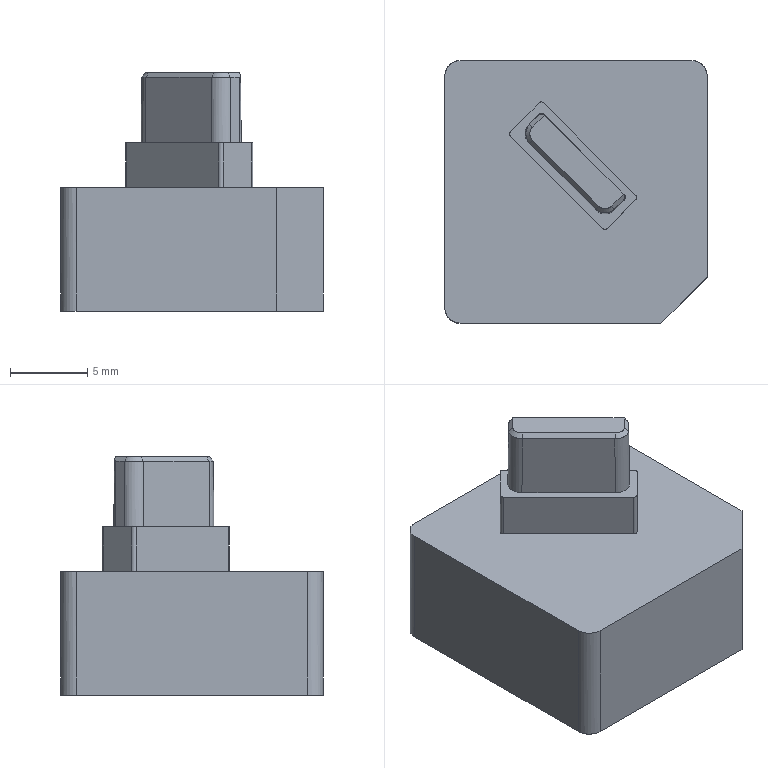NC program | PowerMill | posted with a generic post | part box 17 x 17 x 15.424 mm
Lines 3638 to 4701 of 38437:
N3735 M6
N3736 S18000 M03
N3737 G00 G90 X0.0 Y0.0
N3738 G43 Z10.804 H14
N3739
N3740 G05 P10000 R8
N3741 X1.6651 Y4.8612
N3742 Z0.914
N3743 G01 Z-0.286 F1200.0
N3744 X1.6309 Y4.8241 F2000.0
N3745 X1.5996 Y4.7844
N3746 X1.5716 Y4.7424
N3747 X1.5469 Y4.6983
N3748 X1.5259 Y4.6523
N3749 X1.5085 Y4.6048
N3750 X1.4949 Y4.5561
N3751 X1.4852 Y4.5066
N3752 X1.4795 Y4.4564
N3753 X1.4777 Y4.4059
N3754 X1.4799 Y4.3554
N3755 X1.4861 Y4.3053
N3756 X1.4962 Y4.2558
N3757 X1.5102 Y4.2072
N3758 X1.528 Y4.1599
N3759 X1.5495 Y4.1141
N3760 X1.5745 Y4.0702
N3761 X1.6029 Y4.0284
N3762 X1.6345 Y3.989
N3763 X1.6651 Y3.9561
N3764 X2.7679 Y2.8534
N3765 X3.243 Y2.3784
N3766 X3.6663 Y1.955
N3767 X4.042 Y1.579
N3768 X4.0851 Y1.5357
N3769 X4.1263 Y1.4944
N3770 X4.1663 Y1.4545
N3771 X4.2063 Y1.4146
N3772 X4.2464 Y1.3748
N3773 X4.2865 Y1.335
N3774 X4.3267 Y1.2951
N3775 X4.3667 Y1.2552
N3776 X4.4064 Y1.215
N3777 X4.4458 Y1.1745
N3778 X4.4844 Y1.1333
N3779 X4.5221 Y1.0911
N3780 X4.5658 Y1.0387
N3781 X4.6004 Y0.9942
N3782 X4.6338 Y0.9488
N3783 X4.6663 Y0.9027
N3784 X4.6979 Y0.8559
N3785 X4.742 Y0.7849
N3786 X4.7831 Y0.7112
N3787 X4.8212 Y0.6347
N3788 X4.8561 Y0.5556
N3789 X4.8877 Y0.4741
N3790 X4.916 Y0.3903
N3791 X4.9408 Y0.3043
N3792 X4.9611 Y0.2199
N3793 X4.9776 Y0.1345
N3794 X4.9902 Y0.0482
N3795 X4.9989 Y-0.0387
N3796 X5.0035 Y-0.1261
N3797 X5.0042 Y-0.2138
N3798 X5.0009 Y-0.3015
N3799 X4.9936 Y-0.3891
N3800 X4.9824 Y-0.4762
N3801 X4.9672 Y-0.5628
N3802 X4.9481 Y-0.6483
N3803 X4.9253 Y-0.7325
N3804 X4.8987 Y-0.8152
N3805 X4.8685 Y-0.8963
N3806 X4.8347 Y-0.9757
N3807 X4.7974 Y-1.0531
N3808 X4.7651 Y-1.1137
N3809 X4.731 Y-1.1732
N3810 X4.6951 Y-1.2317
N3811 X4.6571 Y-1.2887
N3812 X4.6168 Y-1.3442
N3813 X4.5705 Y-1.4027
N3814 X4.516 Y-1.4658
N3815 X4.4657 Y-1.52
N3816 X4.4178 Y-1.5696
N3817 X4.3692 Y-1.6184
N3818 X4.3204 Y-1.6669
N3819 X4.1507 Y-1.8368
N3820 X3.9626 Y-2.0247
N3821 X3.7365 Y-2.2515
N3822 X3.6508 Y-2.3358
N3823 X3.5714 Y-2.4092
N3824 X3.496 Y-2.4741
N3825 X3.4232 Y-2.532
N3826 X3.349 Y-2.5863
N3827 X3.2649 Y-2.6431
N3828 X3.1787 Y-2.6965
N3829 X3.0904 Y-2.7465
N3830 X3.0003 Y-2.7929
N3831 X2.9087 Y-2.8357
N3832 X2.8156 Y-2.8747
N3833 X2.7214 Y-2.9099
N3834 X2.626 Y-2.9413
N3835 X2.6175 Y-2.9439
N3836 X2.5206 Y-2.9711
N3837 X2.4227 Y-2.9945
N3838 X2.3239 Y-3.0141
N3839 X2.2242 Y-3.0297
N3840 X2.1239 Y-3.0414
N3841 X2.023 Y-3.0491
N3842 X1.922 Y-3.0528
N3843 X1.8213 Y-3.0526
N3844 X1.7205 Y-3.0483
N3845 X1.62 Y-3.0401
N3846 X1.5199 Y-3.0278
N3847 X1.4204 Y-3.0116
N3848 X1.3214 Y-2.9915
N3849 X1.2233 Y-2.9675
N3850 X1.1262 Y-2.9396
N3851 X1.0303 Y-2.9078
N3852 X0.9357 Y-2.8723
N3853 X0.8425 Y-2.8331
N3854 X0.751 Y-2.7903
N3855 X0.6629 Y-2.7446
N3856 X0.5766 Y-2.6955
N3857 X0.4919 Y-2.6427
N3858 X0.4088 Y-2.5862
N3859 X0.3273 Y-2.526
N3860 X0.2476 Y-2.4621
N3861 X0.1696 Y-2.3945
N3862 X0.0934 Y-2.3232
N3863 X0.0187 Y-2.2487
N3864 X-0.2458 Y-1.9845
N3865 X-0.5216 Y-1.7085
N3866 X-1.4027 Y-0.8275
N3867 X-3.4423 Y1.2122
N3868 X-3.9342 Y1.7042
N3869 X-4.1355 Y1.9043
N3870 X-4.2178 Y1.9883
N3871 X-4.2906 Y2.0677
N3872 X-4.3559 Y2.1441
N3873 X-4.4146 Y2.2185
N3874 X-4.4688 Y2.2931
N3875 X-4.5263 Y2.3787
N3876 X-4.579 Y2.4639
N3877 X-4.6269 Y2.5488
N3878 X-4.6703 Y2.6334
N3879 X-4.7104 Y2.7195
N3880 X-4.7492 Y2.8111
N3881 X-4.7844 Y2.9043
N3882 X-4.8158 Y2.9981
N3883 X-4.8431 Y3.0922
N3884 X-4.8664 Y3.1863
N3885 X-4.8861 Y3.2806
N3886 X-4.9024 Y3.376
N3887 X-4.9155 Y3.4761
N3888 X-4.9247 Y3.5762
N3889 X-4.9299 Y3.6764
N3890 X-4.9311 Y3.7766
N3891 X-4.9283 Y3.8768
N3892 X-4.9215 Y3.977
N3893 X-4.9106 Y4.0772
N3894 X-4.8958 Y4.1774
N3895 X-4.8772 Y4.2768
N3896 X-4.8548 Y4.3748
N3897 X-4.8288 Y4.4713
N3898 X-4.799 Y4.5663
N3899 X-4.7655 Y4.6599
N3900 X-4.7283 Y4.7523
N3901 X-4.6872 Y4.8434
N3902 X-4.6437 Y4.9311
N3903 X-4.5972 Y5.0168
N3904 X-4.5473 Y5.1009
N3905 X-4.4938 Y5.1835
N3906 X-4.4367 Y5.2646
N3907 X-4.3757 Y5.3441
N3908 X-4.3109 Y5.4221
N3909 X-4.2425 Y5.4984
N3910 X-4.1707 Y5.573
N3911 X-4.0963 Y5.6465
N3912 X-3.9199 Y5.823
N3913 X-3.7245 Y6.0181
N3914 X-3.5679 Y6.1739
N3915 X-3.4512 Y6.2917
N3916 X-3.3847 Y6.357
N3917 X-3.3183 Y6.4169
N3918 X-3.2517 Y6.4718
N3919 X-3.1849 Y6.522
N3920 X-3.1162 Y6.5689
N3921 X-3.0414 Y6.6153
N3922 X-2.9645 Y6.6582
N3923 X-2.8858 Y6.6976
N3924 X-2.8053 Y6.7334
N3925 X-2.7234 Y6.7655
N3926 X-2.6404 Y6.7937
N3927 X-2.5562 Y6.818
N3928 X-2.4711 Y6.8385
N3929 X-2.385 Y6.8552
N3930 X-2.2983 Y6.8678
N3931 X-2.211 Y6.8765
N3932 X-2.1235 Y6.8813
N3933 X-2.0358 Y6.882
N3934 X-1.9482 Y6.8787
N3935 X-1.8609 Y6.8715
N3936 X-1.774 Y6.8603
N3937 X-1.6876 Y6.8451
N3938 X-1.602 Y6.826
N3939 X-1.5173 Y6.8031
N3940 X-1.4338 Y6.7763
N3941 X-1.3515 Y6.7457
N3942 X-1.2708 Y6.7114
N3943 X-1.1917 Y6.6735
N3944 X-1.1144 Y6.632
N3945 X-1.0391 Y6.587
N3946 X-0.9659 Y6.5386
N3947 X-0.8949 Y6.4871
N3948 X-0.8217 Y6.4291
N3949 X-0.7509 Y6.3679
N3950 X-0.6826 Y6.3036
N3951 X-0.616 Y6.2372
N3952 X0.0741 Y5.5471
N3953 X1.6651 Y3.9561
N3954 X1.7023 Y3.9219
N3955 X1.742 Y3.8906
N3956 X1.784 Y3.8626
N3957 X1.8281 Y3.8379
N3958 X1.8741 Y3.8169
N3959 X1.9216 Y3.7995
N3960 X1.9702 Y3.7859
N3961 X2.0198 Y3.7762
N3962 X2.07 Y3.7705
N3963 X2.1205 Y3.7687
N3964 X2.171 Y3.7709
N3965 X2.2211 Y3.7771
N3966 X2.2706 Y3.7872
N3967 X2.3192 Y3.8012
N3968 X2.3665 Y3.819
N3969 X2.4123 Y3.8405
N3970 X2.4562 Y3.8655
N3971 X2.4979 Y3.8939
N3972 X2.5374 Y3.9255
N3973 X2.5702 Y3.9562
N3974 X1.6653 Y4.8614 Z-0.306
N3975 X1.631 Y4.8243
N3976 X1.5997 Y4.7846
N3977 X1.5717 Y4.7425
N3978 X1.5471 Y4.6984
N3979 X1.526 Y4.6524
N3980 X1.5086 Y4.605
N3981 X1.4951 Y4.5563
N3982 X1.4854 Y4.5067
N3983 X1.4796 Y4.4565
N3984 X1.4778 Y4.406
N3985 X1.4801 Y4.3555
N3986 X1.4862 Y4.3054
N3987 X1.4964 Y4.2559
N3988 X1.5104 Y4.2074
N3989 X1.5282 Y4.16
N3990 X1.5497 Y4.1143
N3991 X1.5747 Y4.0704
N3992 X1.603 Y4.0286
N3993 X1.6346 Y3.9892
N3994 X1.6653 Y3.9563
N3995 X3.2373 Y2.3843
N3996 X3.9476 Y1.6739
N3997 X4.4093 Y1.2121
N3998 X4.4759 Y1.1425
N3999 X4.5387 Y1.0712
N4000 X4.5977 Y0.9983
N4001 X4.6528 Y0.9241
N4002 X4.7039 Y0.8485
N4003 X4.7511 Y0.7718
N4004 X4.7943 Y0.6942
N4005 X4.8335 Y0.6156
N4006 X4.8687 Y0.5362
N4007 X4.9 Y0.456
N4008 X4.9276 Y0.3744
N4009 X4.952 Y0.2902
N4010 X4.9724 Y0.2049
N4011 X4.989 Y0.1188
N4012 X5.0017 Y0.0321
N4013 X5.0104 Y-0.0552
N4014 X5.0151 Y-0.1429
N4015 X5.0158 Y-0.2307
N4016 X5.0125 Y-0.3183
N4017 X5.0053 Y-0.4057
N4018 X4.994 Y-0.4927
N4019 X4.9789 Y-0.5791
N4020 X4.9598 Y-0.6646
N4021 X4.9368 Y-0.7492
N4022 X4.91 Y-0.8327
N4023 X4.8797 Y-0.9142
N4024 X4.8456 Y-0.9944
N4025 X4.8076 Y-1.0734
N4026 X4.766 Y-1.151
N4027 X4.7206 Y-1.227
N4028 X4.6716 Y-1.3014
N4029 X4.6191 Y-1.3738
N4030 X4.5631 Y-1.4442
N4031 X4.5175 Y-1.4963
N4032 X4.4612 Y-1.5552
N4033 X4.3802 Y-1.6355
N4034 X4.2991 Y-1.7169
N4035 X4.1088 Y-1.9066
N4036 X3.9524 Y-2.0621
N4037 X3.8343 Y-2.1798
N4038 X3.7519 Y-2.2637
N4039 X3.6744 Y-2.3412
N4040 X3.596 Y-2.4141
N4041 X3.5168 Y-2.4824
N4042 X3.4368 Y-2.5463
N4043 X3.3561 Y-2.6058
N4044 X3.2746 Y-2.6611
N4045 X3.1923 Y-2.7121
N4046 X3.1081 Y-2.76
N4047 X3.0179 Y-2.8067
N4048 X2.9257 Y-2.85
N4049 X2.8316 Y-2.8897
N4050 X2.7358 Y-2.9258
N4051 X2.6409 Y-2.9575
N4052 X2.623 Y-2.9627
N4053 X2.5448 Y-2.9854
N4054 X2.4472 Y-3.0096
N4055 X2.3484 Y-3.0299
N4056 X2.2484 Y-3.0464
N4057 X2.1474 Y-3.0591
N4058 X2.1458 Y-3.0593
N4059 X2.0446 Y-3.0678
N4060 X1.9436 Y-3.0724
N4061 X1.8428 Y-3.073
N4062 X1.7425 Y-3.0697
N4063 X1.6416 Y-3.0623
N4064 X1.5409 Y-3.0509
N4065 X1.4406 Y-3.0356
N4066 X1.3409 Y-3.0163
N4067 X1.242 Y-2.9931
N4068 X1.1443 Y-2.966
N4069 X1.0478 Y-2.9352
N4070 X0.9528 Y-2.9007
N4071 X0.8594 Y-2.8625
N4072 X0.768 Y-2.8208
N4073 X0.6785 Y-2.7756
N4074 X0.5912 Y-2.7271
N4075 X0.5197 Y-2.6838
N4076 X0.4536 Y-2.6412
N4077 X0.3887 Y-2.5968
N4078 X0.3253 Y-2.5504
N4079 X0.2634 Y-2.5019
N4080 X0.1997 Y-2.448
N4081 X0.1325 Y-2.3872
N4082 X0.0754 Y-2.3328
N4083 X0.0192 Y-2.2775
N4084 X-0.0366 Y-2.2219
N4085 X-0.0922 Y-2.1661
N4086 X-0.5381 Y-1.7204
N4087 X-1.0114 Y-1.247
N4088 X-1.8763 Y-0.3821
N4089 X-2.9061 Y0.6478
N4090 X-3.376 Y1.1176
N4091 X-3.6366 Y1.378
N4092 X-3.9395 Y1.6813
N4093 X-4.1637 Y1.9045
N4094 X-4.2385 Y1.9809
N4095 X-4.3092 Y2.0584
N4096 X-4.3758 Y2.137
N4097 X-4.4383 Y2.2169
N4098 X-4.4968 Y2.298
N4099 X-4.5515 Y2.3805
N4100 X-4.6025 Y2.4645
N4101 X-4.65 Y2.5499
N4102 X-4.6943 Y2.6373
N4103 X-4.7368 Y2.7298
N4104 X-4.7756 Y2.8236
N4105 X-4.8105 Y2.9186
N4106 X-4.8416 Y3.0148
N4107 X-4.8689 Y3.1122
N4108 X-4.8924 Y3.2106
N4109 X-4.9119 Y3.3101
N4110 X-4.9275 Y3.41
N4111 X-4.9392 Y3.5105
N4112 X-4.947 Y3.6113
N4113 X-4.9507 Y3.7124
N4114 X-4.9504 Y3.8137
N4115 X-4.9462 Y3.9149
N4116 X-4.9379 Y4.0159
N4117 X-4.9258 Y4.1159
N4118 X-4.9097 Y4.2155
N4119 X-4.8896 Y4.3147
N4120 X-4.8656 Y4.4132
N4121 X-4.8377 Y4.5109
N4122 X-4.8059 Y4.6073
N4123 X-4.7705 Y4.7022
N4124 X-4.7315 Y4.7954
N4125 X-4.6889 Y4.8867
N4126 X-4.6429 Y4.976
N4127 X-4.5936 Y5.0633
N4128 X-4.5409 Y5.1487
N4129 X-4.4847 Y5.2321
N4130 X-4.4249 Y5.3136
N4131 X-4.3616 Y5.3932
N4132 X-4.2946 Y5.4711
N4133 X-4.224 Y5.5472
N4134 X-4.1497 Y5.6217
N4135 X-3.9559 Y5.8152
N4136 X-3.7037 Y6.0674
N4137 X-3.5189 Y6.2528
N4138 X-3.4483 Y6.3241
N4139 X-3.3794 Y6.3892
N4140 X-3.3114 Y6.4485
N4141 X-3.2439 Y6.5023
N4142 X-3.1768 Y6.5511
N4143 X-3.1075 Y6.5968
N4144 X-3.0318 Y6.6422
N4145 X-2.9548 Y6.6838
N4146 X-2.8765 Y6.7215
N4147 X-2.797 Y6.7555
N4148 X-2.7147 Y6.7863
N4149 X-2.631 Y6.8133
N4150 X-2.5463 Y6.8365
N4151 X-2.4606 Y6.8559
N4152 X-2.3742 Y6.8713
N4153 X-2.2872 Y6.8827
N4154 X-2.1999 Y6.8902
N4155 X-2.1125 Y6.8936
N4156 X-2.0251 Y6.8931
N4157 X-1.9378 Y6.8886
N4158 X-1.8509 Y6.8801
N4159 X-1.7646 Y6.8677
N4160 X-1.6792 Y6.8514
N4161 X-1.5948 Y6.8315
N4162 X-1.5115 Y6.8078
N4163 X-1.4293 Y6.7804
N4164 X-1.3481 Y6.7491
N4165 X-1.2682 Y6.714
N4166 X-1.1894 Y6.6751
N4167 X-1.1117 Y6.6324
N4168 X-1.0353 Y6.5858
N4169 X-0.9601 Y6.5352
N4170 X-0.8862 Y6.4807
N4171 X-0.8136 Y6.4223
N4172 X-0.7423 Y6.3599
N4173 X-0.6724 Y6.2935
N4174 X-0.6029 Y6.2245
N4175 X-0.2961 Y5.9175
N4176 X0.0402 Y5.5815
N4177 X0.702 Y4.9196
N4178 X1.6653 Y3.9563
N4179 X1.7024 Y3.922
N4180 X1.7421 Y3.8907
N4181 X1.7841 Y3.8627
N4182 X1.8283 Y3.8381
N4183 X1.8742 Y3.817
N4184 X1.9217 Y3.7996
N4185 X1.9704 Y3.786
N4186 X2.02 Y3.7764
N4187 X2.0702 Y3.7706
N4188 X2.1207 Y3.7688
N4189 X2.1711 Y3.7711
N4190 X2.2213 Y3.7772
N4191 X2.2708 Y3.7874
N4192 X2.3193 Y3.8014
N4193 X2.3666 Y3.8192
N4194 X2.4124 Y3.8406
N4195 X2.4563 Y3.8657
N4196 X2.4981 Y3.894
N4197 X2.5375 Y3.9256
N4198 X2.5704 Y3.9563
N4199 X1.6654 Y4.8615 Z-0.326
N4200 X1.6311 Y4.8244
N4201 X1.5999 Y4.7847
N4202 X1.5718 Y4.7426
N4203 X1.5472 Y4.6985
N4204 X1.5261 Y4.6526
N4205 X1.5087 Y4.6051
N4206 X1.4952 Y4.5564
N4207 X1.4855 Y4.5068
N4208 X1.4797 Y4.4566
N4209 X1.478 Y4.4061
N4210 X1.4802 Y4.3557
N4211 X1.4864 Y4.3055
N4212 X1.4965 Y4.256
N4213 X1.5105 Y4.2075
N4214 X1.5283 Y4.1601
N4215 X1.5498 Y4.1144
N4216 X1.5748 Y4.0705
N4217 X1.6032 Y4.0287
N4218 X1.6348 Y3.9893
N4219 X1.6654 Y3.9564
N4220 X3.2072 Y2.4146
N4221 X4.4096 Y1.2122
N4222 X4.4732 Y1.1459
N4223 X4.5352 Y1.0755
N4224 X4.5951 Y1.0016
N4225 X4.6519 Y0.9251
N4226 X4.7049 Y0.8472
N4227 X4.7537 Y0.7687
N4228 X4.7971 Y0.6916
N4229 X4.8369 Y0.6131
N4230 X4.8731 Y0.5329
N4231 X4.9057 Y0.4513
N4232 X4.9344 Y0.3683
N4233 X4.9594 Y0.284
N4234 X4.9804 Y0.1988
N4235 X4.9976 Y0.1128
N4236 X5.0108 Y0.0261
N4237 X5.0201 Y-0.0611
N4238 X5.0254 Y-0.1485
N4239 X5.0267 Y-0.2361
N4240 X5.024 Y-0.3236
N4241 X5.0173 Y-0.4109
N4242 X5.0067 Y-0.4978
N4243 X4.9921 Y-0.5841
N4244 X4.9736 Y-0.6698
N4245 X4.9512 Y-0.7546
N4246 X4.9249 Y-0.8384
N4247 X4.8948 Y-0.921
N4248 X4.8611 Y-1.0021
N4249 X4.8241 Y-1.0806
N4250 X4.7841 Y-1.1565
N4251 X4.741 Y-1.2297
N4252 X4.695 Y-1.3001
N4253 X4.6593 Y-1.3504
N4254 X4.6225 Y-1.3998
N4255 X4.5844 Y-1.4483
N4256 X4.5446 Y-1.4953
N4257 X4.5028 Y-1.5408
N4258 X4.4597 Y-1.585
N4259 X4.416 Y-1.6286
N4260 X4.3722 Y-1.6721
N4261 X4.3285 Y-1.7157
N4262 X3.9182 Y-2.1256
N4263 X3.7525 Y-2.2925
N4264 X3.6789 Y-2.3649
N4265 X3.602 Y-2.4357
N4266 X3.5236 Y-2.5029
N4267 X3.4453 Y-2.565
N4268 X3.3677 Y-2.6219
N4269 X3.288 Y-2.6758
N4270 X3.2063 Y-2.7268
N4271 X3.1183 Y-2.7771
N4272 X3.0284 Y-2.8239
N4273 X2.9367 Y-2.8672
N4274 X2.8432 Y-2.9069
N4275 X2.7482 Y-2.9428
N4276 X2.6518 Y-2.9751
N4277 X2.6285 Y-2.9818
N4278 X2.5541 Y-3.0035
N4279 X2.4554 Y-3.0281
N4280 X2.3557 Y-3.0488
N4281 X2.2969 Y-3.0591
N4282 X2.1959 Y-3.0737
N4283 X2.0945 Y-3.0842
N4284 X1.9929 Y-3.0907
N4285 X1.8911 Y-3.0933
N4286 X1.7894 Y-3.0918
N4287 X1.6898 Y-3.0865
N4288 X1.5894 Y-3.0771
N4289 X1.4885 Y-3.0636
N4290 X1.3877 Y-3.0462
N4291 X1.2876 Y-3.0248
N4292 X1.1888 Y-2.9997
N4293 X1.092 Y-2.9709
N4294 X0.9975 Y-2.9388
N4295 X0.9044 Y-2.903
N4296 X0.8109 Y-2.8628
N4297 X0.719 Y-2.819
N4298 X0.6289 Y-2.7716
N4299 X0.5408 Y-2.7207
N4300 X0.4548 Y-2.6665
N4301 X0.3711 Y-2.6089
N4302 X0.2898 Y-2.5482
N4303 X0.211 Y-2.4843
N4304 X0.1348 Y-2.4174
N4305 X0.0613 Y-2.3476
N4306 X-0.0107 Y-2.2761
N4307 X-0.3148 Y-1.9719
N4308 X-3.1526 Y0.8658
N4309 X-3.6366 Y1.3497
N4310 X-4.0275 Y1.7411
N4311 X-4.1916 Y1.9048
N4312 X-4.2668 Y1.9824
N4313 X-4.3374 Y2.0607
N4314 X-4.4035 Y2.1399
N4315 X-4.4652 Y2.2197
N4316 X-4.5225 Y2.3003
N4317 X-4.5759 Y2.3821
N4318 X-4.6286 Y2.4702
N4319 X-4.6777 Y2.5599
N4320 X-4.7231 Y2.6512
N4321 X-4.7648 Y2.7438
N4322 X-4.8026 Y2.8377
N4323 X-4.8366 Y2.9327
N4324 X-4.8668 Y3.0286
N4325 X-4.893 Y3.1254
N4326 X-4.9153 Y3.223
N4327 X-4.9343 Y3.3239
N4328 X-4.9493 Y3.4254
N4329 X-4.9604 Y3.5273
N4330 X-4.9675 Y3.6293
N4331 X-4.9706 Y3.7313
N4332 X-4.9696 Y3.8331
N4333 X-4.9647 Y3.9344
N4334 X-4.9559 Y4.0352
N4335 X-4.9431 Y4.1353
N4336 X-4.9264 Y4.2346
N4337 X-4.9055 Y4.3347
N4338 X-4.8808 Y4.4337
N4339 X-4.8523 Y4.5314
N4340 X-4.82 Y4.6277
N4341 X-4.7842 Y4.7223
N4342 X-4.7446 Y4.8153
N4343 X-4.7014 Y4.9067
N4344 X-4.6546 Y4.9965
N4345 X-4.6041 Y5.0846
N4346 X-4.5502 Y5.1708
N4347 X-4.4928 Y5.255
N4348 X-4.432 Y5.3371
N4349 X-4.3679 Y5.4168
N4350 X-4.3006 Y5.4942
N4351 X-4.2303 Y5.5689
N4352 X-4.1578 Y5.6418
N4353 X-3.8673 Y5.9321
N4354 X-3.6285 Y6.1708
N4355 X-3.5084 Y6.2924
N4356 X-3.4366 Y6.3634
N4357 X-3.3683 Y6.4259
N4358 X-3.3023 Y6.4814
N4359 X-3.2371 Y6.5315
N4360 X-3.1645 Y6.5822
N4361 X-3.0903 Y6.6293
N4362 X-3.0145 Y6.6726
N4363 X-2.9373 Y6.7122
N4364 X-2.859 Y6.7479
N4365 X-2.7791 Y6.78
N4366 X-2.6961 Y6.8092
N4367 X-2.612 Y6.8345
N4368 X-2.5267 Y6.856
N4369 X-2.4406 Y6.8736
N4370 X-2.3538 Y6.8872
N4371 X-2.2664 Y6.8969
N4372 X-2.1788 Y6.9026
N4373 X-2.091 Y6.9043
N4374 X-2.0032 Y6.9021
N4375 X-1.9157 Y6.8958
N4376 X-1.8286 Y6.8856
N4377 X-1.742 Y6.8714
N4378 X-1.6581 Y6.8537
N4379 X-1.5748 Y6.8321
N4380 X-1.492 Y6.8065
N4381 X-1.4096 Y6.7769
N4382 X-1.3279 Y6.7434
N4383 X-1.2469 Y6.7058
N4384 X-1.1668 Y6.6643
N4385 X-1.0878 Y6.6188
N4386 X-1.0101 Y6.5695
N4387 X-0.9337 Y6.5163
N4388 X-0.8589 Y6.4594
N4389 X-0.786 Y6.3989
N4390 X-0.7151 Y6.335
N4391 X-0.6463 Y6.2678
N4392 X-0.3122 Y5.934
N4393 X0.2446 Y5.3772
N4394 X1.6654 Y3.9564
N4395 X1.7025 Y3.9221
N4396 X1.7422 Y3.8909
N4397 X1.7843 Y3.8628
N4398 X1.8284 Y3.8382
N4399 X1.8744 Y3.8171
N4400 X1.9218 Y3.7997
N4401 X1.9705 Y3.7862
N4402 X2.0201 Y3.7765
N4403 X2.0703 Y3.7707
N4404 X2.1208 Y3.769
N4405 X2.1712 Y3.7712
N4406 X2.2214 Y3.7774
N4407 X2.2709 Y3.7875
N4408 X2.3194 Y3.8015
N4409 X2.3668 Y3.8193
N4410 X2.4125 Y3.8408
N4411 X2.4564 Y3.8658
N4412 X2.4982 Y3.8942
N4413 X2.5376 Y3.9258
N4414 X2.5705 Y3.9564
N4415 X1.6655 Y4.8616 Z-0.346
N4416 X1.6312 Y4.8245
N4417 X1.6 Y4.7848
N4418 X1.572 Y4.7428
N4419 X1.5473 Y4.6986
N4420 X1.5263 Y4.6527
N4421 X1.5089 Y4.6052
N4422 X1.4953 Y4.5565
N4423 X1.4856 Y4.5069
N4424 X1.4799 Y4.4567
N4425 X1.4781 Y4.4063
N4426 X1.4803 Y4.3558
N4427 X1.4865 Y4.3057
N4428 X1.4966 Y4.2562
N4429 X1.5106 Y4.2076
N4430 X1.5284 Y4.1603
N4431 X1.5499 Y4.1145
N4432 X1.5749 Y4.0706
N4433 X1.6033 Y4.0288
N4434 X1.6349 Y3.9894
N4435 X1.6655 Y3.9565
N4436 X1.7801 Y3.842
N4437 X4.3061 Y1.3159
N4438 X4.4099 Y1.2122
N4439 X4.4748 Y1.1444
N4440 X4.5372 Y1.0736
N4441 X4.5968 Y1.0
N4442 X4.6531 Y0.924
N4443 X4.706 Y0.846
N4444 X4.7553 Y0.7662
N4445 X4.8009 Y0.685
N4446 X4.8426 Y0.6026
N4447 X4.8802 Y0.5195
N4448 X4.9132 Y0.4373
N4449 X4.9424 Y0.3543
N4450 X4.9676 Y0.2704
N4451 X4.9888 Y0.1861
N4452 X5.0061 Y0.1014
N4453 X5.0193 Y0.0166
N4454 X5.0287 Y-0.0687
N4455 X5.0344 Y-0.1569
N4456 X5.0361 Y-0.2451
N4457 X5.0338 Y-0.3333
N4458 X5.0275 Y-0.4211
N4459 X5.0173 Y-0.5084
N4460 X5.0031 Y-0.595
N4461 X4.9851 Y-0.6808
N4462 X4.9631 Y-0.7654
N4463 X4.9374 Y-0.8489
N4464 X4.9079 Y-0.9312
N4465 X4.8748 Y-1.0119
N4466 X4.839 Y-1.0889
N4467 X4.8007 Y-1.1623
N4468 X4.7632 Y-1.2273
N4469 X4.7236 Y-1.291
N4470 X4.6816 Y-1.3532
N4471 X4.6371 Y-1.4136
N4472 X4.5854 Y-1.4776
N4473 X4.5333 Y-1.5368
N4474 X4.4817 Y-1.5915
N4475 X4.4288 Y-1.6448
N4476 X4.3751 Y-1.6973
N4477 X4.2524 Y-1.8194
N4478 X4.1039 Y-1.9686
N4479 X3.9581 Y-2.1134
N4480 X3.7839 Y-2.2878
N4481 X3.7074 Y-2.3647
N4482 X3.6306 Y-2.437
N4483 X3.5531 Y-2.5047
N4484 X3.4749 Y-2.5678
N4485 X3.3958 Y-2.6268
N4486 X3.3116 Y-2.6844
N4487 X3.2251 Y-2.7388
N4488 X3.1365 Y-2.7898
N4489 X3.0458 Y-2.8375
N4490 X2.9532 Y-2.8815
N4491 X2.8588 Y-2.9221
N4492 X2.7647 Y-2.9582
N4493 X2.669 Y-2.9907
N4494 X2.6342 Y-3.001
N4495 X2.5717 Y-3.0195
N4496 X2.4728 Y-3.0446
N4497 X2.4068 Y-3.0591
N4498 X2.3059 Y-3.0779
N4499 X2.2049 Y-3.0927
N4500 X2.1039 Y-3.1035
N4501 X2.0028 Y-3.1103
N4502 X1.9008 Y-3.1132
N4503 X1.7988 Y-3.112
N4504 X1.6969 Y-3.1069
N4505 X1.5952 Y-3.0978
N4506 X1.494 Y-3.0848
N4507 X1.3933 Y-3.0677
N4508 X1.2934 Y-3.0468
N4509 X1.1944 Y-3.022
N4510 X1.0965 Y-2.9933
N4511 X0.9998 Y-2.9608
N4512 X0.9045 Y-2.9246
N4513 X0.8107 Y-2.8846
N4514 X0.7186 Y-2.8411
N4515 X0.6282 Y-2.7939
N4516 X0.5397 Y-2.7433
N4517 X0.468 Y-2.6988
N4518 X0.3977 Y-2.6522
N4519 X0.329 Y-2.6032
N4520 X0.2621 Y-2.5518
N4521 X0.1898 Y-2.4918
N4522 X0.1188 Y-2.4287
N4523 X0.0572 Y-2.3708
N4524 X-0.0033 Y-2.3117
N4525 X-0.063 Y-2.2519
N4526 X-0.2815 Y-2.0335
N4527 X-0.5262 Y-1.7887
N4528 X-1.0538 Y-1.2611
N4529 X-2.2657 Y-0.0493
N4530 X-3.5272 Y1.2122
N4531 X-4.161 Y1.8458
N4532 X-4.2341 Y1.9189
N4533 X-4.3052 Y1.9937
N4534 X-4.3732 Y2.071
N4535 X-4.438 Y2.1508
N4536 X-4.4996 Y2.2328
N4537 X-4.5578 Y2.317
N4538 X-4.6125 Y2.4032
N4539 X-4.6637 Y2.4913
N4540 X-4.7113 Y2.5812
N4541 X-4.7553 Y2.6727
N4542 X-4.7957 Y2.7658
N4543 X-4.8326 Y2.8612
N4544 X-4.8658 Y2.9579
N4545 X-4.8952 Y3.0558
N4546 X-4.9207 Y3.1548
N4547 X-4.9423 Y3.2546
N4548 X-4.96 Y3.3551
N4549 X-4.9738 Y3.4563
N4550 X-4.9835 Y3.5579
N4551 X-4.9893 Y3.6598
N4552 X-4.9911 Y3.7619
N4553 X-4.9889 Y3.864
N4554 X-4.9827 Y3.9659
N4555 X-4.9725 Y4.0675
N4556 X-4.9583 Y4.1687
N4557 X-4.9402 Y4.2691
N4558 X-4.9182 Y4.3687
N4559 X-4.8923 Y4.4673
N4560 X-4.8626 Y4.5649
N4561 X-4.8291 Y4.6613
N4562 X-4.7919 Y4.7562
N4563 X-4.7509 Y4.8497
N4564 X-4.7063 Y4.9415
N4565 X-4.6581 Y5.0316
N4566 X-4.6065 Y5.1196
N4567 X-4.5514 Y5.2056
N4568 X-4.4931 Y5.2893
N4569 X-4.4315 Y5.3706
N4570 X-4.3668 Y5.4495
N4571 X-4.2991 Y5.5258
N4572 X-4.2284 Y5.5994
N4573 X-3.7519 Y6.0758
N4574 X-3.6038 Y6.2237
N4575 X-3.5218 Y6.3074
N4576 X-3.456 Y6.373
N4577 X-3.3887 Y6.4345
N4578 X-3.3199 Y6.4921
N4579 X-3.2499 Y6.5457
N4580 X-3.1787 Y6.5952
N4581 X-3.1064 Y6.6408
N4582 X-3.0301 Y6.6841
N4583 X-2.9518 Y6.724
N4584 X-2.8718 Y6.7602
N4585 X-2.7903 Y6.7928
N4586 X-2.7074 Y6.8215
N4587 X-2.6234 Y6.8465
N4588 X-2.5382 Y6.8676
N4589 X-2.4522 Y6.8849
N4590 X-2.3656 Y6.8981
N4591 X-2.2784 Y6.9075
N4592 X-2.1909 Y6.9128
N4593 X-2.1032 Y6.9142
N4594 X-2.0155 Y6.9115
N4595 X-1.9281 Y6.9049
N4596 X-1.8411 Y6.8942
N4597 X-1.7546 Y6.8797
N4598 X-1.67 Y6.8615
N4599 X-1.5869 Y6.8398
N4600 X-1.5047 Y6.8145
N4601 X-1.4232 Y6.7853
N4602 X-1.3425 Y6.7522
N4603 X-1.2624 Y6.715
N4604 X-1.183 Y6.6738
N4605 X-1.1045 Y6.6289
N4606 X-1.0214 Y6.5768
N4607 X-0.9418 Y6.5224
N4608 X-0.8656 Y6.4656
N4609 X-0.8044 Y6.4156
N4610 X-0.7384 Y6.3567
N4611 X-0.6627 Y6.2845
N4612 X-0.5609 Y6.1831
N4613 X-0.3815 Y6.0036
N4614 X1.6655 Y3.9565
N4615 X1.7026 Y3.9222
N4616 X1.7423 Y3.891
N4617 X1.7844 Y3.863
N4618 X1.8285 Y3.8383
N4619 X1.8745 Y3.8172
N4620 X1.9219 Y3.7999
N4621 X1.9706 Y3.7863
N4622 X2.0202 Y3.7766
N4623 X2.0704 Y3.7709
N4624 X2.1209 Y3.7691
N4625 X2.1714 Y3.7713
N4626 X2.2215 Y3.7775
N4627 X2.271 Y3.7876
N4628 X2.3195 Y3.8016
N4629 X2.3669 Y3.8194
N4630 X2.4126 Y3.8409
N4631 X2.4565 Y3.8659
N4632 X2.4983 Y3.8943
N4633 X2.5377 Y3.9259
N4634 X2.5706 Y3.9565
N4635 X1.6657 Y4.8617 Z-0.366
N4636 X1.6314 Y4.8246
N4637 X1.6001 Y4.7849
N4638 X1.5721 Y4.7429
N4639 X1.5475 Y4.6988
N4640 X1.5264 Y4.6528
N4641 X1.509 Y4.6053
N4642 X1.4954 Y4.5567
N4643 X1.4857 Y4.5071
N4644 X1.48 Y4.4569
N4645 X1.4782 Y4.4064
N4646 X1.4804 Y4.3559
N4647 X1.4866 Y4.3058
N4648 X1.4967 Y4.2563
N4649 X1.5107 Y4.2077
N4650 X1.5285 Y4.1604
N4651 X1.55 Y4.1146
N4652 X1.575 Y4.0707
N4653 X1.6034 Y4.0289
N4654 X1.635 Y3.9895
N4655 X1.6657 Y3.9566
N4656 X4.4101 Y1.2122
N4657 X4.4757 Y1.1437
N4658 X4.5382 Y1.0728
N4659 X4.5975 Y0.9995
N4660 X4.6535 Y0.9239
N4661 X4.706 Y0.8463
N4662 X4.7551 Y0.7667
N4663 X4.8008 Y0.6851
N4664 X4.8437 Y0.6008
N4665 X4.8823 Y0.5163
N4666 X4.9166 Y0.4318
N4667 X4.9467 Y0.3474
N4668 X4.9726 Y0.2631
N4669 X4.9943 Y0.179
N4670 X5.0119 Y0.0953
N4671 X5.0256 Y0.011
N4672 X5.036 Y-0.0771
N4673 X5.0424 Y-0.1652
N4674 X5.0448 Y-0.2531
N4675 X5.0432 Y-0.3406
N4676 X5.0377 Y-0.4275
N4677 X5.0282 Y-0.5138
N4678 X5.0147 Y-0.5995
N4679 X4.9972 Y-0.6859
N4680 X4.9758 Y-0.7713
N4681 X4.9506 Y-0.8554
N4682 X4.9216 Y-0.9381
N4683 X4.889 Y-1.0192
N4684 X4.8528 Y-1.0986
N4685 X4.813 Y-1.1761
N4686 X4.7698 Y-1.2517
N4687 X4.7234 Y-1.3253
N4688 X4.6755 Y-1.3942
N4689 X4.6284 Y-1.4558
N4690 X4.5784 Y-1.515
N4691 X4.5195 Y-1.5792
N4692 X4.4435 Y-1.657
N4693 X4.3562 Y-1.7443
N4694 X4.0983 Y-2.0022
N4695 X3.8423 Y-2.2576
N4696 X3.7519 Y-2.3486
N4697 X3.6779 Y-2.4207
N4698 X3.6011 Y-2.4899
N4699 X3.5219 Y-2.5559
N4700 X3.4404 Y-2.6187
N4701 X3.3566 Y-2.6782
N4702 X3.2707 Y-2.7343
N4703 X3.1828 Y-2.7869
N4704 X3.0932 Y-2.8359
N4705 X3.0018 Y-2.8813
N4706 X2.9089 Y-2.9231
N4707 X2.8144 Y-2.9611
N4708 X2.7182 Y-2.9956
N4709 X2.6402 Y-3.0201
N4710 X2.6203 Y-3.0264
N4711 X2.521 Y-3.0535
N4712 X2.4975 Y-3.0593
N4713 X2.3979 Y-3.0814
N4714 X2.2973 Y-3.0997
N4715 X2.1959 Y-3.114
N4716 X2.0939 Y-3.1244
N4717 X1.9914 Y-3.1308
N4718 X1.8887 Y-3.1332
N4719 X1.7861 Y-3.1316
N4720 X1.6836 Y-3.126
N4721 X1.5817 Y-3.1165
N4722 X1.4803 Y-3.103
N4723 X1.3798 Y-3.0856
N4724 X1.2803 Y-3.0643
N4725 X1.1817 Y-3.0392
N4726 X1.0839 Y-3.0103
N4727 X0.9882 Y-2.9779
N4728 X0.8947 Y-2.942
N4729 X0.8029 Y-2.9028
N4730 X0.7144 Y-2.8614
N4731 X0.6341 Y-2.82
N4732 X0.5539 Y-2.7748
N4733 X0.4752 Y-2.7271
N4734 X0.3982 Y-2.6768
N4735 X0.3231 Y-2.6237
N4736 X0.2496 Y-2.5675
N4737 X0.1735 Y-2.5047
N4738 X0.0947 Y-2.4347
N4739 X0.0187 Y-2.3625
N4740 X-0.0522 Y-2.2916
N4741 X-0.1235 Y-2.2194
N4742 X-0.2831 Y-2.0604
N4743 X-0.4348 Y-1.9084
N4744 X-0.7576 Y-1.5855
N4745 X-1.4419 Y-0.9014
N4746 X-3.4056 Y1.0623
N4747 X-4.1291 Y1.7856
N4748 X-4.2139 Y1.8702
N4749 X-4.2932 Y1.9516
N4750 X-4.3626 Y2.0279
N4751 X-4.4243 Y2.1009
N4752 X-4.4818 Y2.1747
N4753 X-4.5425 Y2.2587
N4754 X-4.5996 Y2.3446
N4755 X-4.653 Y2.4319
N4756 X-4.7026 Y2.5207
N4757 X-4.7483 Y2.6108
N4758 X-4.7903 Y2.7021
N4759 X-4.8287 Y2.7949
N4760 X-4.8646 Y2.892
N4761 X-4.8967 Y2.9901
N4762 X-4.9248 Y3.0889
N4763 X-4.9489 Y3.1884
N4764 X-4.9691 Y3.2885
N4765 X-4.9853 Y3.3889
N4766 X-4.9976 Y3.4897
N4767 X-5.0059 Y3.5909
N4768 X-5.0103 Y3.6936
N4769 X-5.0107 Y3.7963
N4770 X-5.0072 Y3.8989
N4771 X-4.9996 Y4.0011
N4772 X-4.9881 Y4.1029
N4773 X-4.9727 Y4.2041
N4774 X-4.9533 Y4.3046
N4775 X-4.93 Y4.4042
N4776 X-4.9028 Y4.503
N4777 X-4.8718 Y4.6006
N4778 X-4.837 Y4.697
N4779 X-4.7984 Y4.792
N4780 X-4.7561 Y4.8856
N4781 X-4.7101 Y4.9775
N4782 X-4.6631 Y5.0634
N4783 X-4.6129 Y5.1474
N4784 X-4.5591 Y5.2301
N4785 X-4.5013 Y5.3118
N4786 X-4.4395 Y5.3924
N4787 X-4.3734 Y5.4719
N4788 X-4.3032 Y5.5505
N4789 X-4.2289 Y5.6278
N4790 X-4.1521 Y5.7043
N4791 X-3.8285 Y6.0272
N4792 X-3.565 Y6.2923
N4793 X-3.5144 Y6.3431
N4794 X-3.4629 Y6.393
N4795 X-3.4075 Y6.444
N4796 X-3.3468 Y6.4958
N4797 X-3.2904 Y6.5399
N4798 X-3.2322 Y6.5815